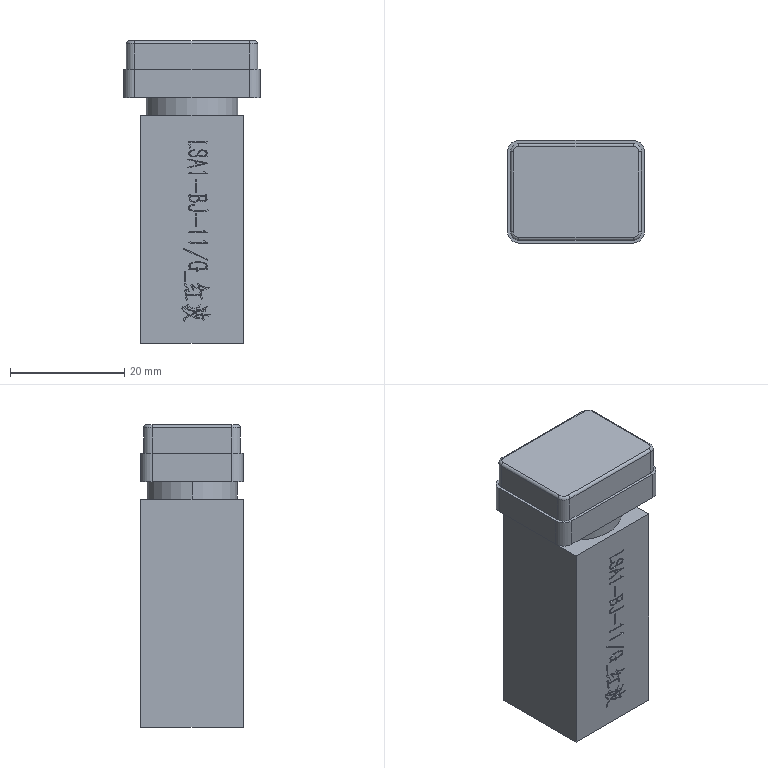Part | STEP file | QA-LSA1-BJ-11 | 1 solid | 400 faces | box 24 x 18 x 53 mm | volume 17646 mm3 | plane 265 | spline 117 | cylinder 14 | torus 4 | commonest cylinder face diameters 1 x4 3 x4 4 x4 16 x2